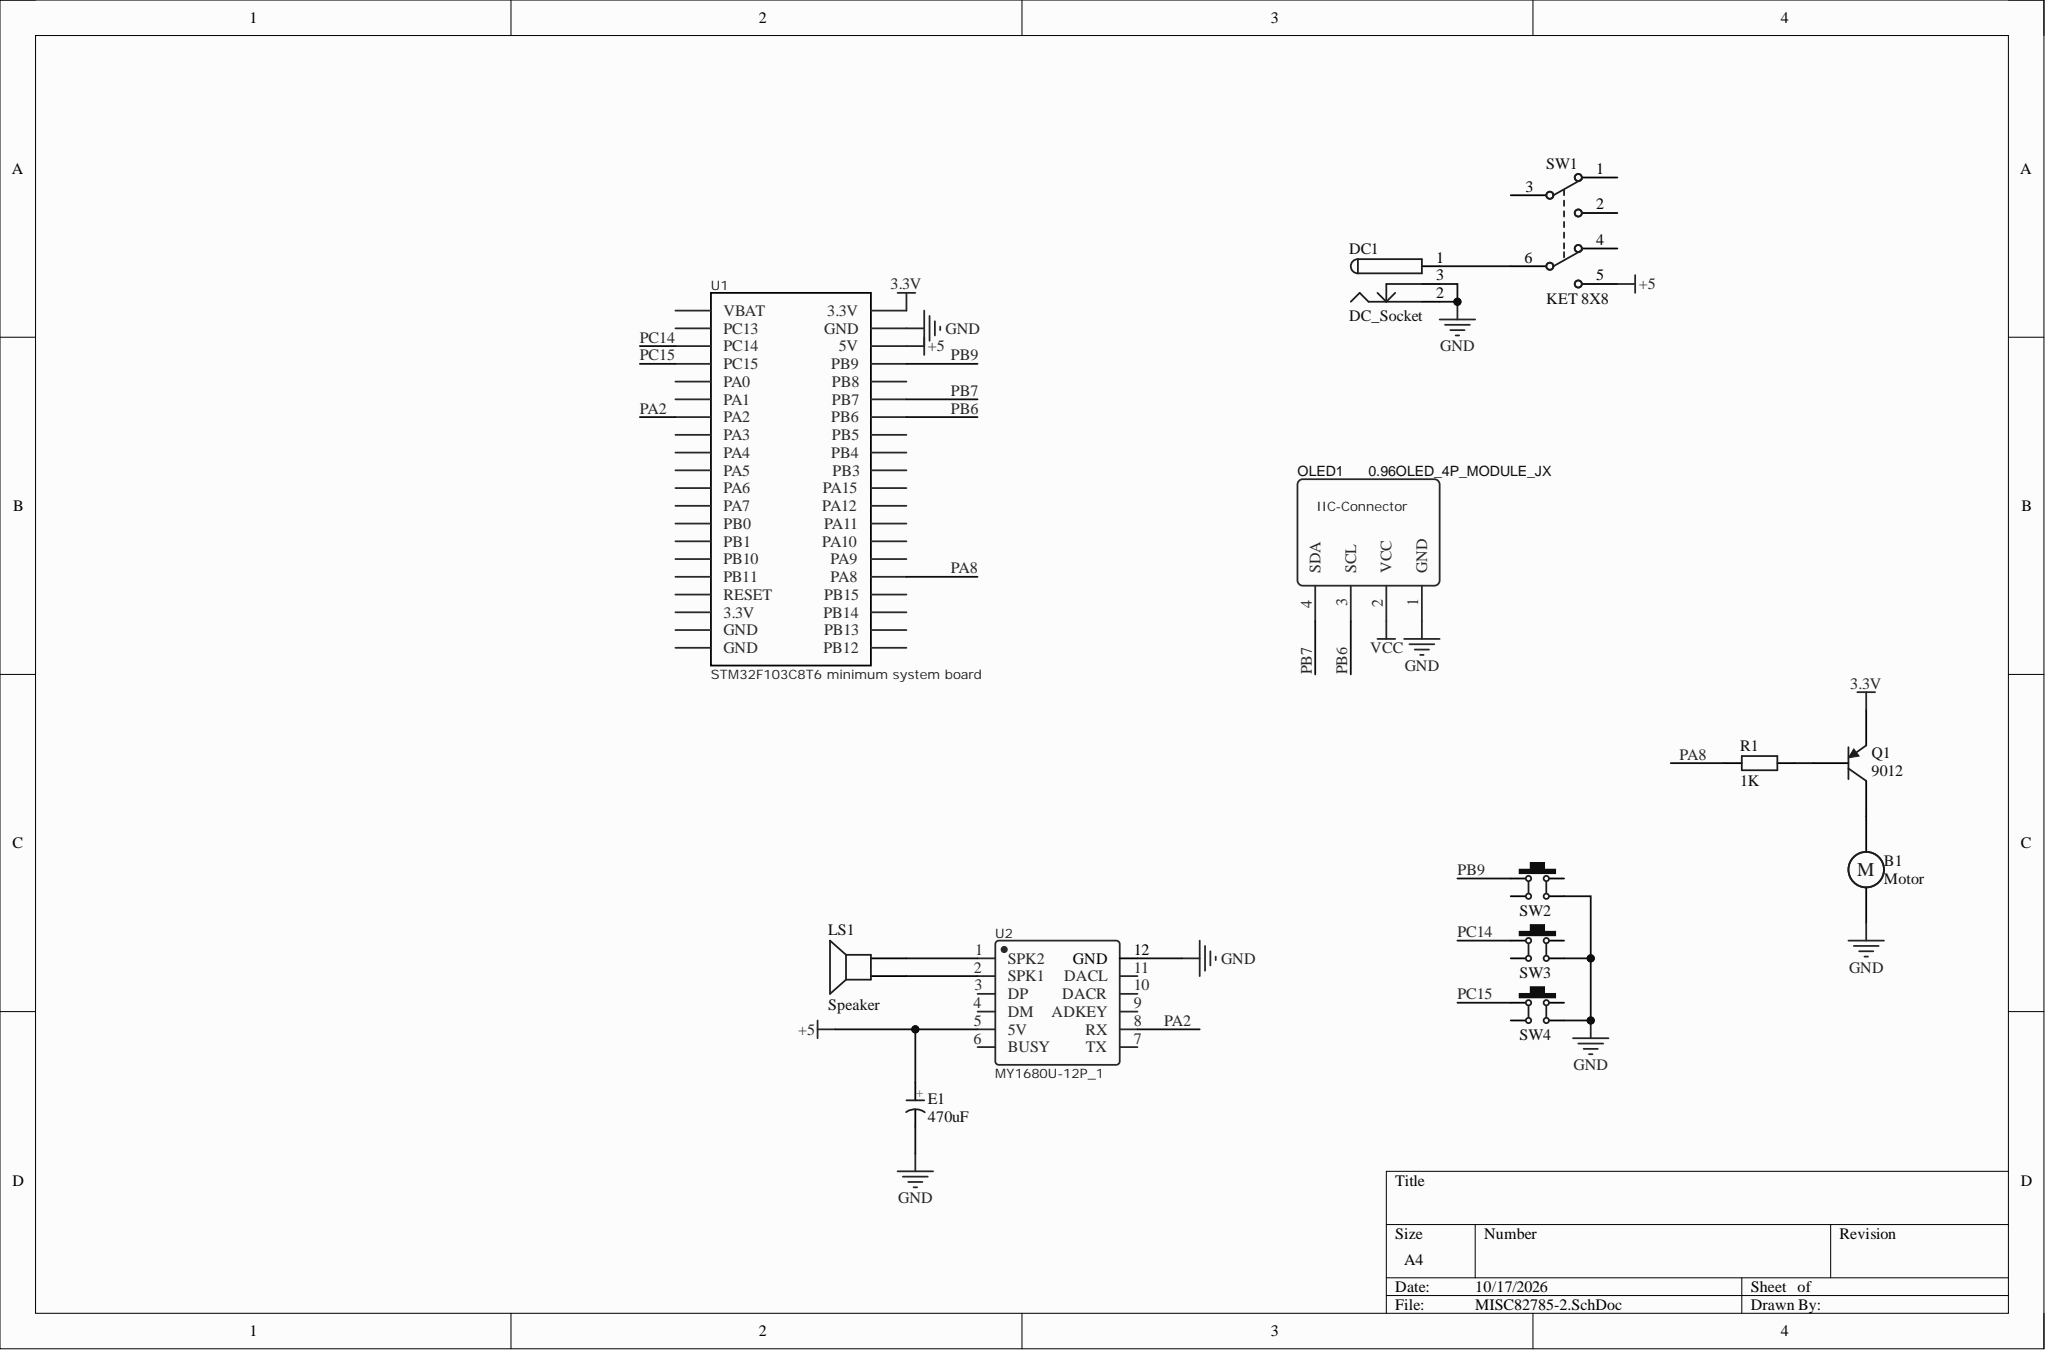Circuit board | Altium Designer | 13 parts | 15 nets
Bill of materials:
Comment,Description,Designator,Footprint,LibRef,Quantity
"Motor","Motor, General Kind","B1","RB5-10.5","Motor","1"
"DC_Socket","","DC1","DC-002","DC_Socket","1"
"470uF","THT solid capacitor","E1","CS 2.0*5*8 - C","CS","1"
"Speaker","Loudspeaker","LS1","PIN2","Speaker","1"
"0.96OLED_4P_MODULE_JX","","OLED1","0.96OLED_4P","0.96OLED_4P_MODULE_JX","1"
"9012","PNP General Purpose Amplifier","Q1","TO-92A","2N3906","1"
"1K","Color-band resistor","R1","RS 1/4W","R-S","1"
"KET 8X8","8*8 self-locking switch","SW1","KFT DIP-8X8","KET 8X8","1"
"6x6x5","THT 6x6 tactile switch","SW2, SW3, SW4","TSW DIP-6*6*6","TSW DIP-6x6","3"
"STM32F103C8T6 minimum system board","","U1","STM32核心板","STM32F103C8T6最小系统板","1"
"MY1680U-12P_1","","U2","COMM-TH_MY1680-12P","MY1680U-12P_1","1"
Netlist (Protel format):
[
B1
RB5-10.5
Motor



]
[
DC1
DC-002
DC_Socket



]
[
E1
CS 2.0*5*8 - C
470uF



]
[
LS1
PIN2
Speaker



]
[
OLED1
0.96OLED_4P
0.96OLED_4P_MODULE_JX



]
[
Q1
TO-92A
9012



]
[
R1
RS 1/4W
1K



]
[
SW1
KFT DIP-8X8
KET 8X8



]
[
SW2
TSW DIP-6*6*6
6x6x5



]
[
SW3
TSW DIP-6*6*6
6x6x5



]
[
SW4
TSW DIP-6*6*6
6x6x5



]
[
U1
STM32核心板
STM32F103C8T6 minimum system board



]
[
U2
COMM-TH_MY1680-12P
MY1680U-12P_1



]
(
PC15
SW4-1
U1-4
)
(
PC14
SW3-1
U1-3
)
(
PB9
SW2-1
U1-37
)
(
PB7
OLED1-4
U1-35
)
(
PB6
OLED1-3
U1-34
)
(
PA8
R1-1
U1-25
)
(
PA2
U1-7
U2-8
)
(
NetQ1_2
Q1-2
R1-2
)
(
NetLS1_2
LS1-2
U2-1
)
(
NetLS1_1
LS1-1
U2-2
)
(
NetDC1_1
DC1-1
SW1-6
)
(
NetB1_1
B1-1
Q1-3
)
(
GND
B1-2
DC1-2
DC1-3
E1-2
OLED1-1
SW2-3
SW3-3
SW4-3
U1-39
U2-12
)
(
+5
E1-1
SW1-5
U1-38
U2-5
)
(
3.3V
Q1-1
U1-40
)